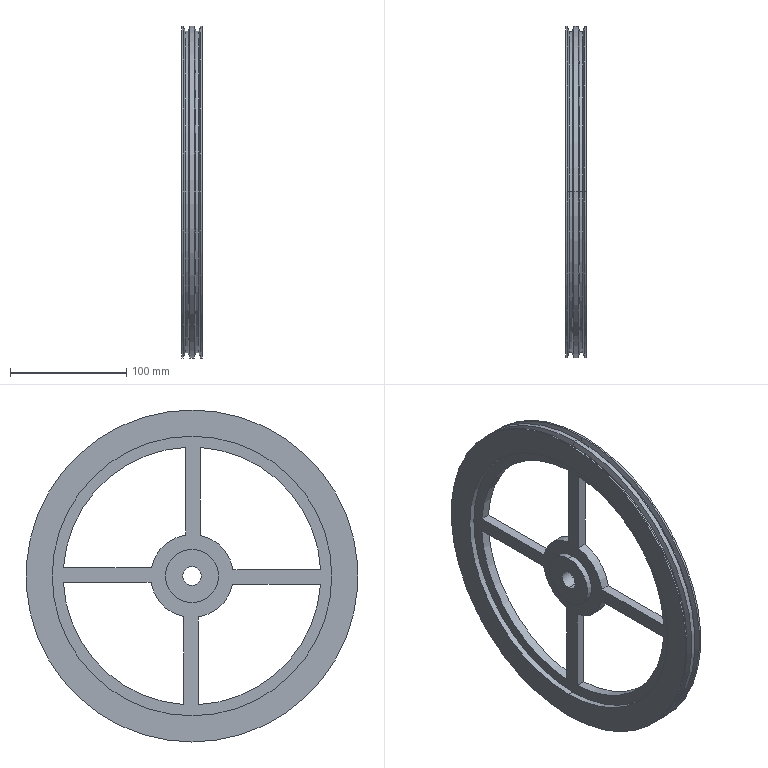Part | SolidWorks | features ICE 6, CirPattern 1, Revolution 1 | 1 solid | 50 faces | box 18 x 285 x 285 mm | volume 431975 mm3 | cylinder 28 | plane 14 | cone 8 | commonest cylinder face diameters 285 x6 45.741 x4 71.176 x4 221.11 x4 240 x4 276.214 x4
STEP:
#1=CARTESIAN_POINT('',(0.,0.,22.87));
#2=VERTEX_POINT('',#1);
#3=CARTESIAN_POINT('',(0.,0.,-22.87));
#4=VERTEX_POINT('',#3);
#5=CARTESIAN_POINT('',(0.,0.,0.));
#6=DIRECTION('',(-1.,0.,0.));
#7=DIRECTION('',(0.,0.,1.));
#8=AXIS2_PLACEMENT_3D('',#5,#6,#7);
#9=CIRCLE('',#8,22.87);
#10=EDGE_CURVE('',#2,#4,#9,.T.);
#11=ORIENTED_EDGE('',*,*,#10,.F.);
#12=CARTESIAN_POINT('',(5.,0.,22.87));
#13=VERTEX_POINT('',#12);
#14=CARTESIAN_POINT('',(0.,0.,22.87));
#15=DIRECTION('',(1.,0.,0.));
#16=VECTOR('',#15,1000.);
#17=LINE('',#14,#16);
#18=EDGE_CURVE('',#2,#13,#17,.T.);
#19=ORIENTED_EDGE('',*,*,#18,.T.);
#20=CARTESIAN_POINT('',(5.,0.,-22.87));
#21=VERTEX_POINT('',#20);
#22=CARTESIAN_POINT('',(5.,0.,0.));
#23=DIRECTION('',(-1.,0.,0.));
#24=DIRECTION('',(0.,0.,1.));
#25=AXIS2_PLACEMENT_3D('',#22,#23,#24);
#26=CIRCLE('',#25,22.87);
#27=EDGE_CURVE('',#13,#21,#26,.T.);
#28=ORIENTED_EDGE('',*,*,#27,.T.);
#29=CARTESIAN_POINT('',(0.,0.,-22.87));
#30=DIRECTION('',(1.,0.,0.));
#31=VECTOR('',#30,1000.);
#32=LINE('',#29,#31);
#33=EDGE_CURVE('',#4,#21,#32,.T.);
#34=ORIENTED_EDGE('',*,*,#33,.F.);
#35=EDGE_LOOP('',(#11,#19,#28,#34));
#36=FACE_OUTER_BOUND('',#35,.T.);
#37=CARTESIAN_POINT('',(0.,0.,0.));
#38=DIRECTION('',(1.,0.,0.));
#39=DIRECTION('',(0.,0.,-1.));
#40=AXIS2_PLACEMENT_3D('',#37,#38,#39);
#41=CYLINDRICAL_SURFACE('',#40,22.87);
#42=ADVANCED_FACE('',(#36),#41,.T.);
#43=CARTESIAN_POINT('',(18.,0.,-22.87));
#44=VERTEX_POINT('',#43);
#45=CARTESIAN_POINT('',(18.,0.,22.87));
#46=VERTEX_POINT('',#45);
#47=CARTESIAN_POINT('',(18.,0.,0.));
#48=DIRECTION('',(1.,0.,0.));
#49=DIRECTION('',(0.,0.,-1.));
#50=AXIS2_PLACEMENT_3D('',#47,#48,#49);
#51=CIRCLE('',#50,22.87);
#52=EDGE_CURVE('',#44,#46,#51,.T.);
#53=ORIENTED_EDGE('',*,*,#52,.F.);
#54=CARTESIAN_POINT('',(13.,0.,-22.87));
#55=VERTEX_POINT('',#54);
#56=CARTESIAN_POINT('',(18.,0.,-22.87));
#57=DIRECTION('',(-1.,0.,0.));
#58=VECTOR('',#57,1000.);
#59=LINE('',#56,#58);
#60=EDGE_CURVE('',#44,#55,#59,.T.);
#61=ORIENTED_EDGE('',*,*,#60,.T.);
#62=CARTESIAN_POINT('',(13.,0.,22.87));
#63=VERTEX_POINT('',#62);
#64=CARTESIAN_POINT('',(13.,0.,0.));
#65=DIRECTION('',(1.,0.,0.));
#66=DIRECTION('',(0.,0.,-1.));
#67=AXIS2_PLACEMENT_3D('',#64,#65,#66);
#68=CIRCLE('',#67,22.87);
#69=EDGE_CURVE('',#55,#63,#68,.T.);
#70=ORIENTED_EDGE('',*,*,#69,.T.);
#71=CARTESIAN_POINT('',(18.,0.,22.87));
#72=DIRECTION('',(-1.,0.,0.));
#73=VECTOR('',#72,1000.);
#74=LINE('',#71,#73);
#75=EDGE_CURVE('',#46,#63,#74,.T.);
#76=ORIENTED_EDGE('',*,*,#75,.F.);
#77=EDGE_LOOP('',(#53,#61,#70,#76));
#78=FACE_OUTER_BOUND('',#77,.T.);
#79=CARTESIAN_POINT('',(18.,0.,0.));
#80=DIRECTION('',(-1.,0.,0.));
#81=DIRECTION('',(0.,0.,1.));
#82=AXIS2_PLACEMENT_3D('',#79,#80,#81);
#83=CYLINDRICAL_SURFACE('',#82,22.87);
#84=ADVANCED_FACE('',(#78),#83,.T.);
#85=CARTESIAN_POINT('',(0.,0.,-8.));
#86=VERTEX_POINT('',#85);
#87=CARTESIAN_POINT('',(0.,0.,8.));
#88=VERTEX_POINT('',#87);
#89=CARTESIAN_POINT('',(0.,0.,0.));
#90=DIRECTION('',(-1.,0.,0.));
#91=DIRECTION('',(0.,0.,1.));
#92=AXIS2_PLACEMENT_3D('',#89,#90,#91);
#93=CIRCLE('',#92,8.);
#94=EDGE_CURVE('',#86,#88,#93,.T.);
#95=ORIENTED_EDGE('',*,*,#94,.T.);
#96=CARTESIAN_POINT('',(18.,0.,8.));
#97=VERTEX_POINT('',#96);
#98=CARTESIAN_POINT('',(0.,0.,8.));
#99=DIRECTION('',(1.,0.,0.));
#100=VECTOR('',#99,1000.);
#101=LINE('',#98,#100);
#102=EDGE_CURVE('',#88,#97,#101,.T.);
#103=ORIENTED_EDGE('',*,*,#102,.T.);
#104=CARTESIAN_POINT('',(18.,0.,-8.));
#105=VERTEX_POINT('',#104);
#106=CARTESIAN_POINT('',(18.,0.,0.));
#107=DIRECTION('',(1.,0.,0.));
#108=DIRECTION('',(0.,0.,-1.));
#109=AXIS2_PLACEMENT_3D('',#106,#107,#108);
#110=CIRCLE('',#109,8.);
#111=EDGE_CURVE('',#97,#105,#110,.T.);
#112=ORIENTED_EDGE('',*,*,#111,.T.);
#113=CARTESIAN_POINT('',(0.,0.,-8.));
#114=DIRECTION('',(1.,0.,0.));
#115=VECTOR('',#114,1000.);
#116=LINE('',#113,#115);
#117=EDGE_CURVE('',#86,#105,#116,.T.);
#118=ORIENTED_EDGE('',*,*,#117,.F.);
#119=EDGE_LOOP('',(#95,#103,#112,#118));
#120=FACE_OUTER_BOUND('',#119,.T.);
#121=CARTESIAN_POINT('',(0.,0.,0.));
#122=DIRECTION('',(1.,0.,0.));
#123=DIRECTION('',(0.,0.,-1.));
#124=AXIS2_PLACEMENT_3D('',#121,#122,#123);
#125=CYLINDRICAL_SURFACE('',#124,8.);
#126=ADVANCED_FACE('',(#120),#125,.F.);
#127=CARTESIAN_POINT('',(13.,0.,120.));
#128=VERTEX_POINT('',#127);
#129=CARTESIAN_POINT('',(13.,0.,-120.));
#130=VERTEX_POINT('',#129);
#131=CARTESIAN_POINT('',(13.,0.,0.));
#132=DIRECTION('',(1.,0.,0.));
#133=DIRECTION('',(0.,0.,-1.));
#134=AXIS2_PLACEMENT_3D('',#131,#132,#133);
#135=CIRCLE('',#134,120.);
#136=EDGE_CURVE('',#128,#130,#135,.T.);
#137=ORIENTED_EDGE('',*,*,#136,.F.);
#138=CARTESIAN_POINT('',(18.,0.,120.));
#139=VERTEX_POINT('',#138);
#140=CARTESIAN_POINT('',(13.,0.,120.));
#141=DIRECTION('',(1.,0.,0.));
#142=VECTOR('',#141,1000.);
#143=LINE('',#140,#142);
#144=EDGE_CURVE('',#128,#139,#143,.T.);
#145=ORIENTED_EDGE('',*,*,#144,.T.);
#146=CARTESIAN_POINT('',(18.,0.,-120.));
#147=VERTEX_POINT('',#146);
#148=CARTESIAN_POINT('',(18.,0.,0.));
#149=DIRECTION('',(1.,0.,0.));
#150=DIRECTION('',(0.,0.,-1.));
#151=AXIS2_PLACEMENT_3D('',#148,#149,#150);
#152=CIRCLE('',#151,120.);
#153=EDGE_CURVE('',#139,#147,#152,.T.);
#154=ORIENTED_EDGE('',*,*,#153,.T.);
#155=CARTESIAN_POINT('',(13.,0.,-120.));
#156=DIRECTION('',(1.,0.,0.));
#157=VECTOR('',#156,1000.);
#158=LINE('',#155,#157);
#159=EDGE_CURVE('',#130,#147,#158,.T.);
#160=ORIENTED_EDGE('',*,*,#159,.F.);
#161=EDGE_LOOP('',(#137,#145,#154,#160));
#162=FACE_OUTER_BOUND('',#161,.T.);
#163=CARTESIAN_POINT('',(13.,0.,0.));
#164=DIRECTION('',(1.,0.,0.));
#165=DIRECTION('',(0.,0.,-1.));
#166=AXIS2_PLACEMENT_3D('',#163,#164,#165);
#167=CYLINDRICAL_SURFACE('',#166,120.);
#168=ADVANCED_FACE('',(#162),#167,.F.);
#169=CARTESIAN_POINT('',(5.,0.,-120.));
#170=VERTEX_POINT('',#169);
#171=CARTESIAN_POINT('',(5.,0.,120.));
#172=VERTEX_POINT('',#171);
#173=CARTESIAN_POINT('',(5.,0.,0.));
#174=DIRECTION('',(-1.,0.,0.));
#175=DIRECTION('',(0.,0.,1.));
#176=AXIS2_PLACEMENT_3D('',#173,#174,#175);
#177=CIRCLE('',#176,120.);
#178=EDGE_CURVE('',#170,#172,#177,.T.);
#179=ORIENTED_EDGE('',*,*,#178,.F.);
#180=CARTESIAN_POINT('',(0.,0.,-120.));
#181=VERTEX_POINT('',#180);
#182=CARTESIAN_POINT('',(5.,0.,-120.));
#183=DIRECTION('',(-1.,0.,0.));
#184=VECTOR('',#183,1000.);
#185=LINE('',#182,#184);
#186=EDGE_CURVE('',#170,#181,#185,.T.);
#187=ORIENTED_EDGE('',*,*,#186,.T.);
#188=CARTESIAN_POINT('',(0.,0.,120.));
#189=VERTEX_POINT('',#188);
#190=CARTESIAN_POINT('',(0.,0.,0.));
#191=DIRECTION('',(-1.,0.,0.));
#192=DIRECTION('',(0.,0.,1.));
#193=AXIS2_PLACEMENT_3D('',#190,#191,#192);
#194=CIRCLE('',#193,120.);
#195=EDGE_CURVE('',#181,#189,#194,.T.);
#196=ORIENTED_EDGE('',*,*,#195,.T.);
#197=CARTESIAN_POINT('',(5.,0.,120.));
#198=DIRECTION('',(-1.,0.,0.));
#199=VECTOR('',#198,1000.);
#200=LINE('',#197,#199);
#201=EDGE_CURVE('',#172,#189,#200,.T.);
#202=ORIENTED_EDGE('',*,*,#201,.F.);
#203=EDGE_LOOP('',(#179,#187,#196,#202));
#204=FACE_OUTER_BOUND('',#203,.T.);
#205=CARTESIAN_POINT('',(5.,0.,0.));
#206=DIRECTION('',(-1.,0.,0.));
#207=DIRECTION('',(0.,0.,1.));
#208=AXIS2_PLACEMENT_3D('',#205,#206,#207);
#209=CYLINDRICAL_SURFACE('',#208,120.);
#210=ADVANCED_FACE('',(#204),#209,.F.);
#211=CARTESIAN_POINT('',(18.,0.,142.5));
#212=VERTEX_POINT('',#211);
#213=CARTESIAN_POINT('',(18.,0.,-142.5));
#214=VERTEX_POINT('',#213);
#215=CARTESIAN_POINT('',(18.,0.,0.));
#216=DIRECTION('',(-1.,0.,0.));
#217=DIRECTION('',(0.,0.,1.));
#218=AXIS2_PLACEMENT_3D('',#215,#216,#217);
#219=CIRCLE('',#218,142.5);
#220=EDGE_CURVE('',#212,#214,#219,.T.);
#221=ORIENTED_EDGE('',*,*,#220,.T.);
#222=CARTESIAN_POINT('',(16.241,0.,-142.5));
#223=VERTEX_POINT('',#222);
#224=CARTESIAN_POINT('',(0.,0.,-142.5));
#225=DIRECTION('',(-1.,0.,0.));
#226=VECTOR('',#225,1000.);
#227=LINE('',#224,#226);
#228=EDGE_CURVE('',#214,#223,#227,.T.);
#229=ORIENTED_EDGE('',*,*,#228,.T.);
#230=CARTESIAN_POINT('',(16.241,0.,142.5));
#231=VERTEX_POINT('',#230);
#232=CARTESIAN_POINT('',(16.241,0.,0.));
#233=DIRECTION('',(-1.,0.,0.));
#234=DIRECTION('',(0.,0.,1.));
#235=AXIS2_PLACEMENT_3D('',#232,#233,#234);
#236=CIRCLE('',#235,142.5);
#237=EDGE_CURVE('',#231,#223,#236,.T.);
#238=ORIENTED_EDGE('',*,*,#237,.F.);
#239=CARTESIAN_POINT('',(0.,0.,142.5));
#240=DIRECTION('',(-1.,0.,0.));
#241=VECTOR('',#240,1000.);
#242=LINE('',#239,#241);
#243=EDGE_CURVE('',#212,#231,#242,.T.);
#244=ORIENTED_EDGE('',*,*,#243,.F.);
#245=EDGE_LOOP('',(#221,#229,#238,#244));
#246=FACE_OUTER_BOUND('',#245,.T.);
#247=CARTESIAN_POINT('',(0.,0.,0.));
#248=DIRECTION('',(-1.,0.,0.));
#249=DIRECTION('',(0.,0.,1.));
#250=AXIS2_PLACEMENT_3D('',#247,#248,#249);
#251=CYLINDRICAL_SURFACE('',#250,142.5);
#252=ADVANCED_FACE('',(#246),#251,.T.);
#253=CARTESIAN_POINT('',(14.915,0.,138.107));
#254=VERTEX_POINT('',#253);
#255=CARTESIAN_POINT('',(14.915,0.,-138.107));
#256=VERTEX_POINT('',#255);
#257=CARTESIAN_POINT('',(14.915,0.,0.));
#258=DIRECTION('',(-1.,0.,0.));
#259=DIRECTION('',(0.,0.,1.));
#260=AXIS2_PLACEMENT_3D('',#257,#258,#259);
#261=CIRCLE('',#260,138.107);
#262=EDGE_CURVE('',#254,#256,#261,.T.);
#263=ORIENTED_EDGE('',*,*,#262,.F.);
#264=CARTESIAN_POINT('',(16.241,0.,142.5));
#265=DIRECTION('',(0.2889,0.,0.9574));
#266=VECTOR('',#265,1000.);
#267=LINE('',#264,#266);
#268=EDGE_CURVE('',#254,#231,#267,.T.);
#269=ORIENTED_EDGE('',*,*,#268,.T.);
#270=ORIENTED_EDGE('',*,*,#237,.T.);
#271=CARTESIAN_POINT('',(16.241,0.,-142.5));
#272=DIRECTION('',(0.2889,0.,-0.9574));
#273=VECTOR('',#272,1000.);
#274=LINE('',#271,#273);
#275=EDGE_CURVE('',#256,#223,#274,.T.);
#276=ORIENTED_EDGE('',*,*,#275,.F.);
#277=EDGE_LOOP('',(#263,#269,#270,#276));
#278=FACE_OUTER_BOUND('',#277,.T.);
#279=CARTESIAN_POINT('',(16.241,0.,0.));
#280=DIRECTION('',(1.,0.,0.));
#281=DIRECTION('',(0.,0.,-1.));
#282=AXIS2_PLACEMENT_3D('',#279,#280,#281);
#283=CONICAL_SURFACE('',#282,142.5,1.278);
#284=ADVANCED_FACE('',(#278),#283,.T.);
#285=ORIENTED_EDGE('',*,*,#262,.T.);
#286=CARTESIAN_POINT('',(12.264,0.,-138.107));
#287=VERTEX_POINT('',#286);
#288=CARTESIAN_POINT('',(0.,0.,-138.107));
#289=DIRECTION('',(-1.,0.,0.));
#290=VECTOR('',#289,1000.);
#291=LINE('',#288,#290);
#292=EDGE_CURVE('',#256,#287,#291,.T.);
#293=ORIENTED_EDGE('',*,*,#292,.T.);
#294=CARTESIAN_POINT('',(12.264,0.,138.107));
#295=VERTEX_POINT('',#294);
#296=CARTESIAN_POINT('',(12.264,0.,0.));
#297=DIRECTION('',(-1.,0.,0.));
#298=DIRECTION('',(0.,0.,1.));
#299=AXIS2_PLACEMENT_3D('',#296,#297,#298);
#300=CIRCLE('',#299,138.107);
#301=EDGE_CURVE('',#295,#287,#300,.T.);
#302=ORIENTED_EDGE('',*,*,#301,.F.);
#303=CARTESIAN_POINT('',(0.,0.,138.107));
#304=DIRECTION('',(-1.,0.,0.));
#305=VECTOR('',#304,1000.);
#306=LINE('',#303,#305);
#307=EDGE_CURVE('',#254,#295,#306,.T.);
#308=ORIENTED_EDGE('',*,*,#307,.F.);
#309=EDGE_LOOP('',(#285,#293,#302,#308));
#310=FACE_OUTER_BOUND('',#309,.T.);
#311=CARTESIAN_POINT('',(0.,0.,0.));
#312=DIRECTION('',(-1.,0.,0.));
#313=DIRECTION('',(0.,0.,1.));
#314=AXIS2_PLACEMENT_3D('',#311,#312,#313);
#315=CYLINDRICAL_SURFACE('',#314,138.107);
#316=ADVANCED_FACE('',(#310),#315,.T.);
#317=ORIENTED_EDGE('',*,*,#301,.T.);
#318=CARTESIAN_POINT('',(11.013,0.,-142.5));
#319=VERTEX_POINT('',#318);
#320=CARTESIAN_POINT('',(12.264,0.,-138.107));
#321=DIRECTION('',(-0.2741,0.,-0.9617));
#322=VECTOR('',#321,1000.);
#323=LINE('',#320,#322);
#324=EDGE_CURVE('',#287,#319,#323,.T.);
#325=ORIENTED_EDGE('',*,*,#324,.T.);
#326=CARTESIAN_POINT('',(11.013,0.,142.5));
#327=VERTEX_POINT('',#326);
#328=CARTESIAN_POINT('',(11.013,0.,0.));
#329=DIRECTION('',(-1.,0.,0.));
#330=DIRECTION('',(0.,0.,1.));
#331=AXIS2_PLACEMENT_3D('',#328,#329,#330);
#332=CIRCLE('',#331,142.5);
#333=EDGE_CURVE('',#327,#319,#332,.T.);
#334=ORIENTED_EDGE('',*,*,#333,.F.);
#335=CARTESIAN_POINT('',(12.264,0.,138.107));
#336=DIRECTION('',(-0.2741,0.,0.9617));
#337=VECTOR('',#336,1000.);
#338=LINE('',#335,#337);
#339=EDGE_CURVE('',#295,#327,#338,.T.);
#340=ORIENTED_EDGE('',*,*,#339,.F.);
#341=EDGE_LOOP('',(#317,#325,#334,#340));
#342=FACE_OUTER_BOUND('',#341,.T.);
#343=CARTESIAN_POINT('',(12.264,0.,0.));
#344=DIRECTION('',(-1.,0.,0.));
#345=DIRECTION('',(0.,0.,1.));
#346=AXIS2_PLACEMENT_3D('',#343,#344,#345);
#347=CONICAL_SURFACE('',#346,138.107,1.293);
#348=ADVANCED_FACE('',(#342),#347,.T.);
#349=ORIENTED_EDGE('',*,*,#333,.T.);
#350=CARTESIAN_POINT('',(7.11,0.,-142.5));
#351=VERTEX_POINT('',#350);
#352=CARTESIAN_POINT('',(0.,0.,-142.5));
#353=DIRECTION('',(-1.,0.,0.));
#354=VECTOR('',#353,1000.);
#355=LINE('',#352,#354);
#356=EDGE_CURVE('',#319,#351,#355,.T.);
#357=ORIENTED_EDGE('',*,*,#356,.T.);
#358=CARTESIAN_POINT('',(7.11,0.,142.5));
#359=VERTEX_POINT('',#358);
#360=CARTESIAN_POINT('',(7.11,0.,0.));
#361=DIRECTION('',(-1.,0.,0.));
#362=DIRECTION('',(0.,0.,1.));
#363=AXIS2_PLACEMENT_3D('',#360,#361,#362);
#364=CIRCLE('',#363,142.5);
#365=EDGE_CURVE('',#359,#351,#364,.T.);
#366=ORIENTED_EDGE('',*,*,#365,.F.);
#367=CARTESIAN_POINT('',(0.,0.,142.5));
#368=DIRECTION('',(-1.,0.,0.));
#369=VECTOR('',#368,1000.);
#370=LINE('',#367,#369);
#371=EDGE_CURVE('',#327,#359,#370,.T.);
#372=ORIENTED_EDGE('',*,*,#371,.F.);
#373=EDGE_LOOP('',(#349,#357,#366,#372));
#374=FACE_OUTER_BOUND('',#373,.T.);
#375=CARTESIAN_POINT('',(0.,0.,0.));
#376=DIRECTION('',(-1.,0.,0.));
#377=DIRECTION('',(0.,0.,1.));
#378=AXIS2_PLACEMENT_3D('',#375,#376,#377);
#379=CYLINDRICAL_SURFACE('',#378,142.5);
#380=ADVANCED_FACE('',(#374),#379,.T.);
#381=CARTESIAN_POINT('',(5.784,0.,138.107));
#382=VERTEX_POINT('',#381);
#383=CARTESIAN_POINT('',(5.784,0.,-138.107));
#384=VERTEX_POINT('',#383);
#385=CARTESIAN_POINT('',(5.784,0.,0.));
#386=DIRECTION('',(-1.,0.,0.));
#387=DIRECTION('',(0.,0.,1.));
#388=AXIS2_PLACEMENT_3D('',#385,#386,#387);
#389=CIRCLE('',#388,138.107);
#390=EDGE_CURVE('',#382,#384,#389,.T.);
#391=ORIENTED_EDGE('',*,*,#390,.F.);
#392=CARTESIAN_POINT('',(7.11,0.,142.5));
#393=DIRECTION('',(0.2889,0.,0.9574));
#394=VECTOR('',#393,1000.);
#395=LINE('',#392,#394);
#396=EDGE_CURVE('',#382,#359,#395,.T.);
#397=ORIENTED_EDGE('',*,*,#396,.T.);
#398=ORIENTED_EDGE('',*,*,#365,.T.);
#399=CARTESIAN_POINT('',(7.11,0.,-142.5));
#400=DIRECTION('',(0.2889,0.,-0.9574));
#401=VECTOR('',#400,1000.);
#402=LINE('',#399,#401);
#403=EDGE_CURVE('',#384,#351,#402,.T.);
#404=ORIENTED_EDGE('',*,*,#403,.F.);
#405=EDGE_LOOP('',(#391,#397,#398,#404));
#406=FACE_OUTER_BOUND('',#405,.T.);
#407=CARTESIAN_POINT('',(7.11,0.,0.));
#408=DIRECTION('',(1.,0.,0.));
#409=DIRECTION('',(0.,0.,-1.));
#410=AXIS2_PLACEMENT_3D('',#407,#408,#409);
#411=CONICAL_SURFACE('',#410,142.5,1.278);
#412=ADVANCED_FACE('',(#406),#411,.T.);
#413=ORIENTED_EDGE('',*,*,#390,.T.);
#414=CARTESIAN_POINT('',(3.207,0.,-138.107));
#415=VERTEX_POINT('',#414);
#416=CARTESIAN_POINT('',(0.,0.,-138.107));
#417=DIRECTION('',(-1.,0.,0.));
#418=VECTOR('',#417,1000.);
#419=LINE('',#416,#418);
#420=EDGE_CURVE('',#384,#415,#419,.T.);
#421=ORIENTED_EDGE('',*,*,#420,.T.);
#422=CARTESIAN_POINT('',(3.207,0.,138.107));
#423=VERTEX_POINT('',#422);
#424=CARTESIAN_POINT('',(3.207,0.,0.));
#425=DIRECTION('',(-1.,0.,0.));
#426=DIRECTION('',(0.,0.,1.));
#427=AXIS2_PLACEMENT_3D('',#424,#425,#426);
#428=CIRCLE('',#427,138.107);
#429=EDGE_CURVE('',#423,#415,#428,.T.);
#430=ORIENTED_EDGE('',*,*,#429,.F.);
#431=CARTESIAN_POINT('',(0.,0.,138.107));
#432=DIRECTION('',(-1.,0.,0.));
#433=VECTOR('',#432,1000.);
#434=LINE('',#431,#433);
#435=EDGE_CURVE('',#382,#423,#434,.T.);
#436=ORIENTED_EDGE('',*,*,#435,.F.);
#437=EDGE_LOOP('',(#413,#421,#430,#436));
#438=FACE_OUTER_BOUND('',#437,.T.);
#439=CARTESIAN_POINT('',(0.,0.,0.));
#440=DIRECTION('',(-1.,0.,0.));
#441=DIRECTION('',(0.,0.,1.));
#442=AXIS2_PLACEMENT_3D('',#439,#440,#441);
#443=CYLINDRICAL_SURFACE('',#442,138.107);
#444=ADVANCED_FACE('',(#438),#443,.T.);
#445=ORIENTED_EDGE('',*,*,#429,.T.);
#446=CARTESIAN_POINT('',(1.44,0.,-142.5));
#447=VERTEX_POINT('',#446);
#448=CARTESIAN_POINT('',(3.207,0.,-138.107));
#449=DIRECTION('',(-0.3732,0.,-0.9277));
#450=VECTOR('',#449,1000.);
#451=LINE('',#448,#450);
#452=EDGE_CURVE('',#415,#447,#451,.T.);
#453=ORIENTED_EDGE('',*,*,#452,.T.);
#454=CARTESIAN_POINT('',(1.44,0.,142.5));
#455=VERTEX_POINT('',#454);
#456=CARTESIAN_POINT('',(1.44,0.,0.));
#457=DIRECTION('',(-1.,0.,0.));
#458=DIRECTION('',(0.,0.,1.));
#459=AXIS2_PLACEMENT_3D('',#456,#457,#458);
#460=CIRCLE('',#459,142.5);
#461=EDGE_CURVE('',#455,#447,#460,.T.);
#462=ORIENTED_EDGE('',*,*,#461,.F.);
#463=CARTESIAN_POINT('',(3.207,0.,138.107));
#464=DIRECTION('',(-0.3732,0.,0.9277));
#465=VECTOR('',#464,1000.);
#466=LINE('',#463,#465);
#467=EDGE_CURVE('',#423,#455,#466,.T.);
#468=ORIENTED_EDGE('',*,*,#467,.F.);
#469=EDGE_LOOP('',(#445,#453,#462,#468));
#470=FACE_OUTER_BOUND('',#469,.T.);
#471=CARTESIAN_POINT('',(3.207,0.,0.));
#472=DIRECTION('',(-1.,0.,0.));
#473=DIRECTION('',(0.,0.,1.));
#474=AXIS2_PLACEMENT_3D('',#471,#472,#473);
#475=CONICAL_SURFACE('',#474,138.107,1.188);
#476=ADVANCED_FACE('',(#470),#475,.T.);
#477=ORIENTED_EDGE('',*,*,#461,.T.);
#478=CARTESIAN_POINT('',(0.,0.,-142.5));
#479=VERTEX_POINT('',#478);
#480=CARTESIAN_POINT('',(0.,0.,-142.5));
#481=DIRECTION('',(-1.,0.,0.));
#482=VECTOR('',#481,1000.);
#483=LINE('',#480,#482);
#484=EDGE_CURVE('',#447,#479,#483,.T.);
#485=ORIENTED_EDGE('',*,*,#484,.T.);
#486=CARTESIAN_POINT('',(0.,0.,142.5));
#487=VERTEX_POINT('',#486);
#488=CARTESIAN_POINT('',(0.,0.,0.));
#489=DIRECTION('',(-1.,0.,0.));
#490=DIRECTION('',(0.,0.,1.));
#491=AXIS2_PLACEMENT_3D('',#488,#489,#490);
#492=CIRCLE('',#491,142.5);
#493=EDGE_CURVE('',#487,#479,#492,.T.);
#494=ORIENTED_EDGE('',*,*,#493,.F.);
#495=CARTESIAN_POINT('',(0.,0.,142.5));
#496=DIRECTION('',(-1.,0.,0.));
#497=VECTOR('',#496,1000.);
#498=LINE('',#495,#497);
#499=EDGE_CURVE('',#455,#487,#498,.T.);
#500=ORIENTED_EDGE('',*,*,#499,.F.);
#501=EDGE_LOOP('',(#477,#485,#494,#500));
#502=FACE_OUTER_BOUND('',#501,.T.);
#503=CARTESIAN_POINT('',(0.,0.,0.));
#504=DIRECTION('',(-1.,0.,0.));
#505=DIRECTION('',(0.,0.,1.));
#506=AXIS2_PLACEMENT_3D('',#503,#504,#505);
#507=CYLINDRICAL_SURFACE('',#506,142.5);
#508=ADVANCED_FACE('',(#502),#507,.T.);
#509=CARTESIAN_POINT('',(5.,-7.038,34.885));
#510=VERTEX_POINT('',#509);
#511=CARTESIAN_POINT('',(5.,-35.176,5.402));
#512=VERTEX_POINT('',#511);
#513=CARTESIAN_POINT('',(5.,0.,0.));
#514=DIRECTION('',(1.,0.,0.));
#515=DIRECTION('',(0.,0.,-1.));
#516=AXIS2_PLACEMENT_3D('',#513,#514,#515);
#517=CIRCLE('',#516,35.588);
#518=EDGE_CURVE('',#510,#512,#517,.T.);
#519=ORIENTED_EDGE('',*,*,#518,.F.);
#520=CARTESIAN_POINT('',(5.,-7.038,110.331));
#521=VERTEX_POINT('',#520);
#522=CARTESIAN_POINT('',(5.,-7.038,34.885));
#523=DIRECTION('',(0.,0.,-1.));
#524=VECTOR('',#523,1000.);
#525=LINE('',#522,#524);
#526=EDGE_CURVE('',#521,#510,#525,.T.);
#527=ORIENTED_EDGE('',*,*,#526,.F.);
#528=CARTESIAN_POINT('',(5.,-110.423,5.402));
#529=VERTEX_POINT('',#528);
#530=CARTESIAN_POINT('',(5.,0.,0.));
#531=DIRECTION('',(-1.,0.,0.));
#532=DIRECTION('',(0.,0.,-1.));
#533=AXIS2_PLACEMENT_3D('',#530,#531,#532);
#534=CIRCLE('',#533,110.555);
#535=EDGE_CURVE('',#529,#521,#534,.T.);
#536=ORIENTED_EDGE('',*,*,#535,.F.);
#537=CARTESIAN_POINT('',(5.,-35.176,5.402));
#538=DIRECTION('',(0.,-1.,0.));
#539=VECTOR('',#538,1000.);
#540=LINE('',#537,#539);
#541=EDGE_CURVE('',#512,#529,#540,.T.);
#542=ORIENTED_EDGE('',*,*,#541,.F.);
#543=EDGE_LOOP('',(#519,#527,#536,#542));
#544=FACE_BOUND('',#543,.T.);
#545=CARTESIAN_POINT('',(5.,34.885,7.038));
#546=VERTEX_POINT('',#545);
#547=CARTESIAN_POINT('',(5.,5.402,35.176));
#548=VERTEX_POINT('',#547);
#549=CARTESIAN_POINT('',(5.,0.,0.));
#550=DIRECTION('',(1.,0.,0.));
#551=DIRECTION('',(0.,-1.,0.));
#552=AXIS2_PLACEMENT_3D('',#549,#550,#551);
#553=CIRCLE('',#552,35.588);
#554=EDGE_CURVE('',#546,#548,#553,.T.);
#555=ORIENTED_EDGE('',*,*,#554,.F.);
#556=CARTESIAN_POINT('',(5.,110.331,7.038));
#557=VERTEX_POINT('',#556);
#558=CARTESIAN_POINT('',(5.,34.885,7.038));
#559=DIRECTION('',(0.,-1.,0.));
#560=VECTOR('',#559,1000.);
#561=LINE('',#558,#560);
#562=EDGE_CURVE('',#557,#546,#561,.T.);
#563=ORIENTED_EDGE('',*,*,#562,.F.);
#564=CARTESIAN_POINT('',(5.,5.402,110.423));
#565=VERTEX_POINT('',#564);
#566=CARTESIAN_POINT('',(5.,0.,0.));
#567=DIRECTION('',(-1.,0.,0.));
#568=DIRECTION('',(0.,-1.,0.));
#569=AXIS2_PLACEMENT_3D('',#566,#567,#568);
#570=CIRCLE('',#569,110.555);
#571=EDGE_CURVE('',#565,#557,#570,.T.);
#572=ORIENTED_EDGE('',*,*,#571,.F.);
#573=CARTESIAN_POINT('',(5.,5.402,35.176));
#574=DIRECTION('',(0.,0.,1.));
#575=VECTOR('',#574,1000.);
#576=LINE('',#573,#575);
#577=EDGE_CURVE('',#548,#565,#576,.T.);
#578=ORIENTED_EDGE('',*,*,#577,.F.);
#579=EDGE_LOOP('',(#555,#563,#572,#578));
#580=FACE_BOUND('',#579,.T.);
#581=CARTESIAN_POINT('',(5.,-34.885,-7.038));
#582=VERTEX_POINT('',#581);
#583=CARTESIAN_POINT('',(5.,-5.402,-35.176));
#584=VERTEX_POINT('',#583);
#585=CARTESIAN_POINT('',(5.,0.,0.));
#586=DIRECTION('',(1.,0.,0.));
#587=DIRECTION('',(0.,1.,0.));
#588=AXIS2_PLACEMENT_3D('',#585,#586,#587);
#589=CIRCLE('',#588,35.588);
#590=EDGE_CURVE('',#582,#584,#589,.T.);
#591=ORIENTED_EDGE('',*,*,#590,.F.);
#592=CARTESIAN_POINT('',(5.,-110.331,-7.038));
#593=VERTEX_POINT('',#592);
#594=CARTESIAN_POINT('',(5.,-34.885,-7.038));
#595=DIRECTION('',(0.,1.,0.));
#596=VECTOR('',#595,1000.);
#597=LINE('',#594,#596);
#598=EDGE_CURVE('',#593,#582,#597,.T.);
#599=ORIENTED_EDGE('',*,*,#598,.F.);
#600=CARTESIAN_POINT('',(5.,-5.402,-110.423));
#601=VERTEX_POINT('',#600);
#602=CARTESIAN_POINT('',(5.,0.,0.));
#603=DIRECTION('',(-1.,0.,0.));
#604=DIRECTION('',(0.,1.,0.));
#605=AXIS2_PLACEMENT_3D('',#602,#603,#604);
#606=CIRCLE('',#605,110.555);
#607=EDGE_CURVE('',#601,#593,#606,.T.);
#608=ORIENTED_EDGE('',*,*,#607,.F.);
#609=CARTESIAN_POINT('',(5.,-5.402,-35.176));
#610=DIRECTION('',(0.,0.,-1.));
#611=VECTOR('',#610,1000.);
#612=LINE('',#609,#611);
#613=EDGE_CURVE('',#584,#601,#612,.T.);
#614=ORIENTED_EDGE('',*,*,#613,.F.);
#615=EDGE_LOOP('',(#591,#599,#608,#614));
#616=FACE_BOUND('',#615,.T.);
#617=CARTESIAN_POINT('',(5.,7.038,-34.885));
#618=VERTEX_POINT('',#617);
#619=CARTESIAN_POINT('',(5.,35.176,-5.402));
#620=VERTEX_POINT('',#619);
#621=CARTESIAN_POINT('',(5.,0.,0.));
#622=DIRECTION('',(1.,0.,0.));
#623=DIRECTION('',(0.,0.,1.));
#624=AXIS2_PLACEMENT_3D('',#621,#622,#623);
#625=CIRCLE('',#624,35.588);
#626=EDGE_CURVE('',#618,#620,#625,.T.);
#627=ORIENTED_EDGE('',*,*,#626,.F.);
#628=CARTESIAN_POINT('',(5.,7.038,-110.331));
#629=VERTEX_POINT('',#628);
#630=CARTESIAN_POINT('',(5.,7.038,-34.885));
#631=DIRECTION('',(0.,0.,1.));
#632=VECTOR('',#631,1000.);
#633=LINE('',#630,#632);
#634=EDGE_CURVE('',#629,#618,#633,.T.);
#635=ORIENTED_EDGE('',*,*,#634,.F.);
#636=CARTESIAN_POINT('',(5.,110.423,-5.402));
#637=VERTEX_POINT('',#636);
#638=CARTESIAN_POINT('',(5.,0.,0.));
#639=DIRECTION('',(-1.,0.,0.));
#640=DIRECTION('',(0.,0.,1.));
#641=AXIS2_PLACEMENT_3D('',#638,#639,#640);
#642=CIRCLE('',#641,110.555);
#643=EDGE_CURVE('',#637,#629,#642,.T.);
#644=ORIENTED_EDGE('',*,*,#643,.F.);
#645=CARTESIAN_POINT('',(5.,35.176,-5.402));
#646=DIRECTION('',(0.,1.,0.));
#647=VECTOR('',#646,1000.);
#648=LINE('',#645,#647);
#649=EDGE_CURVE('',#620,#637,#648,.T.);
#650=ORIENTED_EDGE('',*,*,#649,.F.);
#651=EDGE_LOOP('',(#627,#635,#644,#650));
#652=FACE_BOUND('',#651,.T.);
#653=CARTESIAN_POINT('',(5.,0.,0.));
#654=DIRECTION('',(-1.,0.,0.));
#655=DIRECTION('',(0.,0.,1.));
#656=AXIS2_PLACEMENT_3D('',#653,#654,#655);
#657=CIRCLE('',#656,120.);
#658=EDGE_CURVE('',#172,#170,#657,.T.);
#659=ORIENTED_EDGE('',*,*,#658,.T.);
#660=ORIENTED_EDGE('',*,*,#178,.T.);
#661=EDGE_LOOP('',(#659,#660));
#662=FACE_OUTER_BOUND('',#661,.T.);
#663=CARTESIAN_POINT('',(5.,0.,0.));
#664=DIRECTION('',(-1.,0.,0.));
#665=DIRECTION('',(0.,0.,1.));
#666=AXIS2_PLACEMENT_3D('',#663,#664,#665);
#667=CIRCLE('',#666,22.87);
#668=EDGE_CURVE('',#21,#13,#667,.T.);
#669=ORIENTED_EDGE('',*,*,#668,.F.);
#670=ORIENTED_EDGE('',*,*,#27,.F.);
#671=EDGE_LOOP('',(#669,#670));
#672=FACE_BOUND('',#671,.T.);
#673=CARTESIAN_POINT('',(5.,0.,0.));
#674=DIRECTION('',(-1.,0.,0.));
#675=DIRECTION('',(0.,0.,1.));
#676=AXIS2_PLACEMENT_3D('',#673,#674,#675);
#677=PLANE('',#676);
#678=ADVANCED_FACE('',(#544,#580,#616,#652,#662,#672),#677,.T.);
#679=CARTESIAN_POINT('',(13.,-35.176,5.402));
#680=VERTEX_POINT('',#679);
#681=CARTESIAN_POINT('',(13.,-7.038,34.885));
#682=VERTEX_POINT('',#681);
#683=CARTESIAN_POINT('',(13.,0.,0.));
#684=DIRECTION('',(-1.,0.,0.));
#685=DIRECTION('',(0.,0.,-1.));
#686=AXIS2_PLACEMENT_3D('',#683,#684,#685);
#687=CIRCLE('',#686,35.588);
#688=EDGE_CURVE('',#680,#682,#687,.T.);
#689=ORIENTED_EDGE('',*,*,#688,.F.);
#690=CARTESIAN_POINT('',(13.,-110.423,5.402));
#691=VERTEX_POINT('',#690);
#692=CARTESIAN_POINT('',(13.,0.,5.402));
#693=DIRECTION('',(0.,1.,0.));
#694=VECTOR('',#693,1000.);
#695=LINE('',#692,#694);
#696=EDGE_CURVE('',#691,#680,#695,.T.);
#697=ORIENTED_EDGE('',*,*,#696,.F.);
#698=CARTESIAN_POINT('',(13.,-7.038,110.331));
#699=VERTEX_POINT('',#698);
#700=CARTESIAN_POINT('',(13.,0.,0.));
#701=DIRECTION('',(1.,0.,0.));
#702=DIRECTION('',(0.,0.,-1.));
#703=AXIS2_PLACEMENT_3D('',#700,#701,#702);
#704=CIRCLE('',#703,110.555);
#705=EDGE_CURVE('',#699,#691,#704,.T.);
#706=ORIENTED_EDGE('',*,*,#705,.F.);
#707=CARTESIAN_POINT('',(13.,-7.038,0.));
#708=DIRECTION('',(0.,0.,1.));
#709=VECTOR('',#708,1000.);
#710=LINE('',#707,#709);
#711=EDGE_CURVE('',#682,#699,#710,.T.);
#712=ORIENTED_EDGE('',*,*,#711,.F.);
#713=EDGE_LOOP('',(#689,#697,#706,#712));
#714=FACE_BOUND('',#713,.T.);
#715=CARTESIAN_POINT('',(13.,5.402,35.176));
#716=VERTEX_POINT('',#715);
#717=CARTESIAN_POINT('',(13.,34.885,7.038));
#718=VERTEX_POINT('',#717);
#719=CARTESIAN_POINT('',(13.,0.,0.));
#720=DIRECTION('',(-1.,0.,0.));
#721=DIRECTION('',(0.,0.,-1.));
#722=AXIS2_PLACEMENT_3D('',#719,#720,#721);
#723=CIRCLE('',#722,35.588);
#724=EDGE_CURVE('',#716,#718,#723,.T.);
#725=ORIENTED_EDGE('',*,*,#724,.F.);
#726=CARTESIAN_POINT('',(13.,5.402,110.423));
#727=VERTEX_POINT('',#726);
#728=CARTESIAN_POINT('',(13.,5.402,0.));
#729=DIRECTION('',(0.,0.,-1.));
#730=VECTOR('',#729,1000.);
#731=LINE('',#728,#730);
#732=EDGE_CURVE('',#727,#716,#731,.T.);
#733=ORIENTED_EDGE('',*,*,#732,.F.);
#734=CARTESIAN_POINT('',(13.,110.331,7.038));
#735=VERTEX_POINT('',#734);
#736=CARTESIAN_POINT('',(13.,0.,0.));
#737=DIRECTION('',(1.,0.,0.));
#738=DIRECTION('',(0.,0.,-1.));
#739=AXIS2_PLACEMENT_3D('',#736,#737,#738);
#740=CIRCLE('',#739,110.555);
#741=EDGE_CURVE('',#735,#727,#740,.T.);
#742=ORIENTED_EDGE('',*,*,#741,.F.);
#743=CARTESIAN_POINT('',(13.,0.,7.038));
#744=DIRECTION('',(0.,1.,0.));
#745=VECTOR('',#744,1000.);
#746=LINE('',#743,#745);
#747=EDGE_CURVE('',#718,#735,#746,.T.);
#748=ORIENTED_EDGE('',*,*,#747,.F.);
#749=EDGE_LOOP('',(#725,#733,#742,#748));
#750=FACE_BOUND('',#749,.T.);
#751=CARTESIAN_POINT('',(13.,-5.402,-35.176));
#752=VERTEX_POINT('',#751);
#753=CARTESIAN_POINT('',(13.,-34.885,-7.038));
#754=VERTEX_POINT('',#753);
#755=CARTESIAN_POINT('',(13.,0.,0.));
#756=DIRECTION('',(-1.,0.,0.));
#757=DIRECTION('',(0.,0.,-1.));
#758=AXIS2_PLACEMENT_3D('',#755,#756,#757);
#759=CIRCLE('',#758,35.588);
#760=EDGE_CURVE('',#752,#754,#759,.T.);
#761=ORIENTED_EDGE('',*,*,#760,.F.);
#762=CARTESIAN_POINT('',(13.,-5.402,-110.423));
#763=VERTEX_POINT('',#762);
#764=CARTESIAN_POINT('',(13.,-5.402,0.));
#765=DIRECTION('',(0.,0.,1.));
#766=VECTOR('',#765,1000.);
#767=LINE('',#764,#766);
#768=EDGE_CURVE('',#763,#752,#767,.T.);
#769=ORIENTED_EDGE('',*,*,#768,.F.);
#770=CARTESIAN_POINT('',(13.,-110.331,-7.038));
#771=VERTEX_POINT('',#770);
#772=CARTESIAN_POINT('',(13.,0.,0.));
#773=DIRECTION('',(1.,0.,0.));
#774=DIRECTION('',(0.,0.,-1.));
#775=AXIS2_PLACEMENT_3D('',#772,#773,#774);
#776=CIRCLE('',#775,110.555);
#777=EDGE_CURVE('',#771,#763,#776,.T.);
#778=ORIENTED_EDGE('',*,*,#777,.F.);
#779=CARTESIAN_POINT('',(13.,0.,-7.038));
#780=DIRECTION('',(0.,-1.,0.));
#781=VECTOR('',#780,1000.);
#782=LINE('',#779,#781);
#783=EDGE_CURVE('',#754,#771,#782,.T.);
#784=ORIENTED_EDGE('',*,*,#783,.F.);
#785=EDGE_LOOP('',(#761,#769,#778,#784));
#786=FACE_BOUND('',#785,.T.);
#787=CARTESIAN_POINT('',(13.,35.176,-5.402));
#788=VERTEX_POINT('',#787);
#789=CARTESIAN_POINT('',(13.,7.038,-34.885));
#790=VERTEX_POINT('',#789);
#791=CARTESIAN_POINT('',(13.,0.,0.));
#792=DIRECTION('',(-1.,0.,0.));
#793=DIRECTION('',(0.,0.,-1.));
#794=AXIS2_PLACEMENT_3D('',#791,#792,#793);
#795=CIRCLE('',#794,35.588);
#796=EDGE_CURVE('',#788,#790,#795,.T.);
#797=ORIENTED_EDGE('',*,*,#796,.F.);
#798=CARTESIAN_POINT('',(13.,110.423,-5.402));
#799=VERTEX_POINT('',#798);
#800=CARTESIAN_POINT('',(13.,0.,-5.402));
#801=DIRECTION('',(0.,-1.,0.));
#802=VECTOR('',#801,1000.);
#803=LINE('',#800,#802);
#804=EDGE_CURVE('',#799,#788,#803,.T.);
#805=ORIENTED_EDGE('',*,*,#804,.F.);
#806=CARTESIAN_POINT('',(13.,7.038,-110.331));
#807=VERTEX_POINT('',#806);
#808=CARTESIAN_POINT('',(13.,0.,0.));
#809=DIRECTION('',(1.,0.,0.));
#810=DIRECTION('',(0.,0.,-1.));
#811=AXIS2_PLACEMENT_3D('',#808,#809,#810);
#812=CIRCLE('',#811,110.555);
#813=EDGE_CURVE('',#807,#799,#812,.T.);
#814=ORIENTED_EDGE('',*,*,#813,.F.);
#815=CARTESIAN_POINT('',(13.,7.038,0.));
#816=DIRECTION('',(0.,0.,-1.));
#817=VECTOR('',#816,1000.);
#818=LINE('',#815,#817);
#819=EDGE_CURVE('',#790,#807,#818,.T.);
#820=ORIENTED_EDGE('',*,*,#819,.F.);
#821=EDGE_LOOP('',(#797,#805,#814,#820));
#822=FACE_BOUND('',#821,.T.);
#823=CARTESIAN_POINT('',(13.,0.,0.));
#824=DIRECTION('',(1.,0.,0.));
#825=DIRECTION('',(0.,0.,-1.));
#826=AXIS2_PLACEMENT_3D('',#823,#824,#825);
#827=CIRCLE('',#826,120.);
#828=EDGE_CURVE('',#130,#128,#827,.T.);
#829=ORIENTED_EDGE('',*,*,#828,.T.);
#830=ORIENTED_EDGE('',*,*,#136,.T.);
#831=EDGE_LOOP('',(#829,#830));
#832=FACE_OUTER_BOUND('',#831,.T.);
#833=CARTESIAN_POINT('',(13.,0.,0.));
#834=DIRECTION('',(1.,0.,0.));
#835=DIRECTION('',(0.,0.,-1.));
#836=AXIS2_PLACEMENT_3D('',#833,#834,#835);
#837=CIRCLE('',#836,22.87);
#838=EDGE_CURVE('',#63,#55,#837,.T.);
#839=ORIENTED_EDGE('',*,*,#838,.F.);
#840=ORIENTED_EDGE('',*,*,#69,.F.);
#841=EDGE_LOOP('',(#839,#840));
#842=FACE_BOUND('',#841,.T.);
#843=CARTESIAN_POINT('',(13.,0.,0.));
#844=DIRECTION('',(1.,0.,0.));
#845=DIRECTION('',(0.,0.,-1.));
#846=AXIS2_PLACEMENT_3D('',#843,#844,#845);
#847=PLANE('',#846);
#848=ADVANCED_FACE('',(#714,#750,#786,#822,#832,#842),#847,.T.);
#849=CARTESIAN_POINT('',(0.,0.,0.));
#850=DIRECTION('',(-1.,0.,0.));
#851=DIRECTION('',(0.,0.,1.));
#852=AXIS2_PLACEMENT_3D('',#849,#850,#851);
#853=CIRCLE('',#852,120.);
#854=EDGE_CURVE('',#189,#181,#853,.T.);
#855=ORIENTED_EDGE('',*,*,#854,.F.);
#856=ORIENTED_EDGE('',*,*,#195,.F.);
#857=EDGE_LOOP('',(#855,#856));
#858=FACE_BOUND('',#857,.T.);
#859=ORIENTED_EDGE('',*,*,#493,.T.);
#860=CARTESIAN_POINT('',(0.,0.,0.));
#861=DIRECTION('',(-1.,0.,0.));
#862=DIRECTION('',(0.,0.,1.));
#863=AXIS2_PLACEMENT_3D('',#860,#861,#862);
#864=CIRCLE('',#863,142.5);
#865=EDGE_CURVE('',#479,#487,#864,.T.);
#866=ORIENTED_EDGE('',*,*,#865,.T.);
#867=EDGE_LOOP('',(#859,#866));
#868=FACE_OUTER_BOUND('',#867,.T.);
#869=CARTESIAN_POINT('',(0.,0.,0.));
#870=DIRECTION('',(1.,0.,0.));
#871=DIRECTION('',(0.,0.,-1.));
#872=AXIS2_PLACEMENT_3D('',#869,#870,#871);
#873=PLANE('',#872);
#874=ADVANCED_FACE('',(#858,#868),#873,.F.);
#875=ORIENTED_EDGE('',*,*,#484,.F.);
#876=CARTESIAN_POINT('',(1.44,0.,0.));
#877=DIRECTION('',(-1.,0.,0.));
#878=DIRECTION('',(0.,0.,1.));
#879=AXIS2_PLACEMENT_3D('',#876,#877,#878);
#880=CIRCLE('',#879,142.5);
#881=EDGE_CURVE('',#447,#455,#880,.T.);
#882=ORIENTED_EDGE('',*,*,#881,.T.);
#883=ORIENTED_EDGE('',*,*,#499,.T.);
#884=ORIENTED_EDGE('',*,*,#865,.F.);
#885=EDGE_LOOP('',(#875,#882,#883,#884));
#886=FACE_OUTER_BOUND('',#885,.T.);
#887=CARTESIAN_POINT('',(0.,0.,0.));
#888=DIRECTION('',(-1.,0.,0.));
#889=DIRECTION('',(0.,0.,1.));
#890=AXIS2_PLACEMENT_3D('',#887,#888,#889);
#891=CYLINDRICAL_SURFACE('',#890,142.5);
#892=ADVANCED_FACE('',(#886),#891,.T.);
#893=ORIENTED_EDGE('',*,*,#452,.F.);
#894=CARTESIAN_POINT('',(3.207,0.,0.));
#895=DIRECTION('',(-1.,0.,0.));
#896=DIRECTION('',(0.,0.,1.));
#897=AXIS2_PLACEMENT_3D('',#894,#895,#896);
#898=CIRCLE('',#897,138.107);
#899=EDGE_CURVE('',#415,#423,#898,.T.);
#900=ORIENTED_EDGE('',*,*,#899,.T.);
#901=ORIENTED_EDGE('',*,*,#467,.T.);
#902=ORIENTED_EDGE('',*,*,#881,.F.);
#903=EDGE_LOOP('',(#893,#900,#901,#902));
#904=FACE_OUTER_BOUND('',#903,.T.);
#905=CARTESIAN_POINT('',(3.207,0.,0.));
#906=DIRECTION('',(-1.,0.,0.));
#907=DIRECTION('',(0.,0.,1.));
#908=AXIS2_PLACEMENT_3D('',#905,#906,#907);
#909=CONICAL_SURFACE('',#908,138.107,1.188);
#910=ADVANCED_FACE('',(#904),#909,.T.);
#911=ORIENTED_EDGE('',*,*,#420,.F.);
#912=CARTESIAN_POINT('',(5.784,0.,0.));
#913=DIRECTION('',(-1.,0.,0.));
#914=DIRECTION('',(0.,0.,1.));
#915=AXIS2_PLACEMENT_3D('',#912,#913,#914);
#916=CIRCLE('',#915,138.107);
#917=EDGE_CURVE('',#384,#382,#916,.T.);
#918=ORIENTED_EDGE('',*,*,#917,.T.);
#919=ORIENTED_EDGE('',*,*,#435,.T.);
#920=ORIENTED_EDGE('',*,*,#899,.F.);
#921=EDGE_LOOP('',(#911,#918,#919,#920));
#922=FACE_OUTER_BOUND('',#921,.T.);
#923=CARTESIAN_POINT('',(0.,0.,0.));
#924=DIRECTION('',(-1.,0.,0.));
#925=DIRECTION('',(0.,0.,1.));
#926=AXIS2_PLACEMENT_3D('',#923,#924,#925);
#927=CYLINDRICAL_SURFACE('',#926,138.107);
#928=ADVANCED_FACE('',(#922),#927,.T.);
#929=ORIENTED_EDGE('',*,*,#396,.F.);
#930=ORIENTED_EDGE('',*,*,#917,.F.);
#931=ORIENTED_EDGE('',*,*,#403,.T.);
#932=CARTESIAN_POINT('',(7.11,0.,0.));
#933=DIRECTION('',(-1.,0.,0.));
#934=DIRECTION('',(0.,0.,1.));
#935=AXIS2_PLACEMENT_3D('',#932,#933,#934);
#936=CIRCLE('',#935,142.5);
#937=EDGE_CURVE('',#351,#359,#936,.T.);
#938=ORIENTED_EDGE('',*,*,#937,.T.);
#939=EDGE_LOOP('',(#929,#930,#931,#938));
#940=FACE_OUTER_BOUND('',#939,.T.);
#941=CARTESIAN_POINT('',(7.11,0.,0.));
#942=DIRECTION('',(1.,0.,0.));
#943=DIRECTION('',(0.,0.,-1.));
#944=AXIS2_PLACEMENT_3D('',#941,#942,#943);
#945=CONICAL_SURFACE('',#944,142.5,1.278);
#946=ADVANCED_FACE('',(#940),#945,.T.);
#947=ORIENTED_EDGE('',*,*,#356,.F.);
#948=CARTESIAN_POINT('',(11.013,0.,0.));
#949=DIRECTION('',(-1.,0.,0.));
#950=DIRECTION('',(0.,0.,1.));
#951=AXIS2_PLACEMENT_3D('',#948,#949,#950);
#952=CIRCLE('',#951,142.5);
#953=EDGE_CURVE('',#319,#327,#952,.T.);
#954=ORIENTED_EDGE('',*,*,#953,.T.);
#955=ORIENTED_EDGE('',*,*,#371,.T.);
#956=ORIENTED_EDGE('',*,*,#937,.F.);
#957=EDGE_LOOP('',(#947,#954,#955,#956));
#958=FACE_OUTER_BOUND('',#957,.T.);
#959=CARTESIAN_POINT('',(0.,0.,0.));
#960=DIRECTION('',(-1.,0.,0.));
#961=DIRECTION('',(0.,0.,1.));
#962=AXIS2_PLACEMENT_3D('',#959,#960,#961);
#963=CYLINDRICAL_SURFACE('',#962,142.5);
#964=ADVANCED_FACE('',(#958),#963,.T.);
#965=ORIENTED_EDGE('',*,*,#324,.F.);
#966=CARTESIAN_POINT('',(12.264,0.,0.));
#967=DIRECTION('',(-1.,0.,0.));
#968=DIRECTION('',(0.,0.,1.));
#969=AXIS2_PLACEMENT_3D('',#966,#967,#968);
#970=CIRCLE('',#969,138.107);
#971=EDGE_CURVE('',#287,#295,#970,.T.);
#972=ORIENTED_EDGE('',*,*,#971,.T.);
#973=ORIENTED_EDGE('',*,*,#339,.T.);
#974=ORIENTED_EDGE('',*,*,#953,.F.);
#975=EDGE_LOOP('',(#965,#972,#973,#974));
#976=FACE_OUTER_BOUND('',#975,.T.);
#977=CARTESIAN_POINT('',(12.264,0.,0.));
#978=DIRECTION('',(-1.,0.,0.));
#979=DIRECTION('',(0.,0.,1.));
#980=AXIS2_PLACEMENT_3D('',#977,#978,#979);
#981=CONICAL_SURFACE('',#980,138.107,1.293);
#982=ADVANCED_FACE('',(#976),#981,.T.);
#983=ORIENTED_EDGE('',*,*,#292,.F.);
#984=CARTESIAN_POINT('',(14.915,0.,0.));
#985=DIRECTION('',(-1.,0.,0.));
#986=DIRECTION('',(0.,0.,1.));
#987=AXIS2_PLACEMENT_3D('',#984,#985,#986);
#988=CIRCLE('',#987,138.107);
#989=EDGE_CURVE('',#256,#254,#988,.T.);
#990=ORIENTED_EDGE('',*,*,#989,.T.);
#991=ORIENTED_EDGE('',*,*,#307,.T.);
#992=ORIENTED_EDGE('',*,*,#971,.F.);
#993=EDGE_LOOP('',(#983,#990,#991,#992));
#994=FACE_OUTER_BOUND('',#993,.T.);
#995=CARTESIAN_POINT('',(0.,0.,0.));
#996=DIRECTION('',(-1.,0.,0.));
#997=DIRECTION('',(0.,0.,1.));
#998=AXIS2_PLACEMENT_3D('',#995,#996,#997);
#999=CYLINDRICAL_SURFACE('',#998,138.107);
#1000=ADVANCED_FACE('',(#994),#999,.T.);
#1001=ORIENTED_EDGE('',*,*,#268,.F.);
#1002=ORIENTED_EDGE('',*,*,#989,.F.);
#1003=ORIENTED_EDGE('',*,*,#275,.T.);
#1004=CARTESIAN_POINT('',(16.241,0.,0.));
#1005=DIRECTION('',(-1.,0.,0.));
#1006=DIRECTION('',(0.,0.,1.));
#1007=AXIS2_PLACEMENT_3D('',#1004,#1005,#1006);
#1008=CIRCLE('',#1007,142.5);
#1009=EDGE_CURVE('',#223,#231,#1008,.T.);
#1010=ORIENTED_EDGE('',*,*,#1009,.T.);
#1011=EDGE_LOOP('',(#1001,#1002,#1003,#1010));
#1012=FACE_OUTER_BOUND('',#1011,.T.);
#1013=CARTESIAN_POINT('',(16.241,0.,0.));
#1014=DIRECTION('',(1.,0.,0.));
#1015=DIRECTION('',(0.,0.,-1.));
#1016=AXIS2_PLACEMENT_3D('',#1013,#1014,#1015);
#1017=CONICAL_SURFACE('',#1016,142.5,1.278);
#1018=ADVANCED_FACE('',(#1012),#1017,.T.);
#1019=ORIENTED_EDGE('',*,*,#228,.F.);
#1020=CARTESIAN_POINT('',(18.,0.,0.));
#1021=DIRECTION('',(-1.,0.,0.));
#1022=DIRECTION('',(0.,0.,1.));
#1023=AXIS2_PLACEMENT_3D('',#1020,#1021,#1022);
#1024=CIRCLE('',#1023,142.5);
#1025=EDGE_CURVE('',#214,#212,#1024,.T.);
#1026=ORIENTED_EDGE('',*,*,#1025,.T.);
#1027=ORIENTED_EDGE('',*,*,#243,.T.);
#1028=ORIENTED_EDGE('',*,*,#1009,.F.);
#1029=EDGE_LOOP('',(#1019,#1026,#1027,#1028));
#1030=FACE_OUTER_BOUND('',#1029,.T.);
#1031=CARTESIAN_POINT('',(0.,0.,0.));
#1032=DIRECTION('',(-1.,0.,0.));
#1033=DIRECTION('',(0.,0.,1.));
#1034=AXIS2_PLACEMENT_3D('',#1031,#1032,#1033);
#1035=CYLINDRICAL_SURFACE('',#1034,142.5);
#1036=ADVANCED_FACE('',(#1030),#1035,.T.);
#1037=CARTESIAN_POINT('',(18.,0.,0.));
#1038=DIRECTION('',(1.,0.,0.));
#1039=DIRECTION('',(0.,0.,-1.));
#1040=AXIS2_PLACEMENT_3D('',#1037,#1038,#1039);
#1041=CIRCLE('',#1040,120.);
#1042=EDGE_CURVE('',#147,#139,#1041,.T.);
#1043=ORIENTED_EDGE('',*,*,#1042,.F.);
#1044=ORIENTED_EDGE('',*,*,#153,.F.);
#1045=EDGE_LOOP('',(#1043,#1044));
#1046=FACE_BOUND('',#1045,.T.);
#1047=ORIENTED_EDGE('',*,*,#220,.F.);
#1048=ORIENTED_EDGE('',*,*,#1025,.F.);
#1049=EDGE_LOOP('',(#1047,#1048));
#1050=FACE_OUTER_BOUND('',#1049,.T.);
#1051=CARTESIAN_POINT('',(18.,0.,-142.5));
#1052=DIRECTION('',(-1.,0.,0.));
#1053=DIRECTION('',(0.,0.,1.));
#1054=AXIS2_PLACEMENT_3D('',#1051,#1052,#1053);
#1055=PLANE('',#1054);
#1056=ADVANCED_FACE('',(#1046,#1050),#1055,.F.);
#1057=ORIENTED_EDGE('',*,*,#186,.F.);
#1058=ORIENTED_EDGE('',*,*,#658,.F.);
#1059=ORIENTED_EDGE('',*,*,#201,.T.);
#1060=ORIENTED_EDGE('',*,*,#854,.T.);
#1061=EDGE_LOOP('',(#1057,#1058,#1059,#1060));
#1062=FACE_OUTER_BOUND('',#1061,.T.);
#1063=CARTESIAN_POINT('',(5.,0.,0.));
#1064=DIRECTION('',(-1.,0.,0.));
#1065=DIRECTION('',(0.,0.,1.));
#1066=AXIS2_PLACEMENT_3D('',#1063,#1064,#1065);
#1067=CYLINDRICAL_SURFACE('',#1066,120.);
#1068=ADVANCED_FACE('',(#1062),#1067,.F.);
#1069=ORIENTED_EDGE('',*,*,#144,.F.);
#1070=ORIENTED_EDGE('',*,*,#828,.F.);
#1071=ORIENTED_EDGE('',*,*,#159,.T.);
#1072=ORIENTED_EDGE('',*,*,#1042,.T.);
#1073=EDGE_LOOP('',(#1069,#1070,#1071,#1072));
#1074=FACE_OUTER_BOUND('',#1073,.T.);
#1075=CARTESIAN_POINT('',(13.,0.,0.));
#1076=DIRECTION('',(1.,0.,0.));
#1077=DIRECTION('',(0.,0.,-1.));
#1078=AXIS2_PLACEMENT_3D('',#1075,#1076,#1077);
#1079=CYLINDRICAL_SURFACE('',#1078,120.);
#1080=ADVANCED_FACE('',(#1074),#1079,.F.);
#1081=ORIENTED_EDGE('',*,*,#102,.F.);
#1082=CARTESIAN_POINT('',(0.,0.,0.));
#1083=DIRECTION('',(-1.,0.,0.));
#1084=DIRECTION('',(0.,0.,1.));
#1085=AXIS2_PLACEMENT_3D('',#1082,#1083,#1084);
#1086=CIRCLE('',#1085,8.);
#1087=EDGE_CURVE('',#88,#86,#1086,.T.);
#1088=ORIENTED_EDGE('',*,*,#1087,.T.);
#1089=ORIENTED_EDGE('',*,*,#117,.T.);
#1090=CARTESIAN_POINT('',(18.,0.,0.));
#1091=DIRECTION('',(1.,0.,0.));
#1092=DIRECTION('',(0.,0.,-1.));
#1093=AXIS2_PLACEMENT_3D('',#1090,#1091,#1092);
#1094=CIRCLE('',#1093,8.);
#1095=EDGE_CURVE('',#105,#97,#1094,.T.);
#1096=ORIENTED_EDGE('',*,*,#1095,.T.);
#1097=EDGE_LOOP('',(#1081,#1088,#1089,#1096));
#1098=FACE_OUTER_BOUND('',#1097,.T.);
#1099=CARTESIAN_POINT('',(0.,0.,0.));
#1100=DIRECTION('',(1.,0.,0.));
#1101=DIRECTION('',(0.,0.,-1.));
#1102=AXIS2_PLACEMENT_3D('',#1099,#1100,#1101);
#1103=CYLINDRICAL_SURFACE('',#1102,8.);
#1104=ADVANCED_FACE('',(#1098),#1103,.F.);
#1105=CARTESIAN_POINT('',(18.,0.,0.));
#1106=DIRECTION('',(1.,0.,0.));
#1107=DIRECTION('',(0.,0.,-1.));
#1108=AXIS2_PLACEMENT_3D('',#1105,#1106,#1107);
#1109=CIRCLE('',#1108,22.87);
#1110=EDGE_CURVE('',#46,#44,#1109,.T.);
#1111=ORIENTED_EDGE('',*,*,#1110,.T.);
#1112=ORIENTED_EDGE('',*,*,#52,.T.);
#1113=EDGE_LOOP('',(#1111,#1112));
#1114=FACE_OUTER_BOUND('',#1113,.T.);
#1115=ORIENTED_EDGE('',*,*,#1095,.F.);
#1116=ORIENTED_EDGE('',*,*,#111,.F.);
#1117=EDGE_LOOP('',(#1115,#1116));
#1118=FACE_BOUND('',#1117,.T.);
#1119=CARTESIAN_POINT('',(18.,0.,0.));
#1120=DIRECTION('',(1.,0.,0.));
#1121=DIRECTION('',(0.,0.,-1.));
#1122=AXIS2_PLACEMENT_3D('',#1119,#1120,#1121);
#1123=PLANE('',#1122);
#1124=ADVANCED_FACE('',(#1114,#1118),#1123,.T.);
#1125=ORIENTED_EDGE('',*,*,#60,.F.);
#1126=ORIENTED_EDGE('',*,*,#1110,.F.);
#1127=ORIENTED_EDGE('',*,*,#75,.T.);
#1128=ORIENTED_EDGE('',*,*,#838,.T.);
#1129=EDGE_LOOP('',(#1125,#1126,#1127,#1128));
#1130=FACE_OUTER_BOUND('',#1129,.T.);
#1131=CARTESIAN_POINT('',(18.,0.,0.));
#1132=DIRECTION('',(-1.,0.,0.));
#1133=DIRECTION('',(0.,0.,1.));
#1134=AXIS2_PLACEMENT_3D('',#1131,#1132,#1133);
#1135=CYLINDRICAL_SURFACE('',#1134,22.87);
#1136=ADVANCED_FACE('',(#1130),#1135,.T.);
#1137=CARTESIAN_POINT('',(0.,0.,0.));
#1138=DIRECTION('',(-1.,0.,0.));
#1139=DIRECTION('',(0.,0.,1.));
#1140=AXIS2_PLACEMENT_3D('',#1137,#1138,#1139);
#1141=CIRCLE('',#1140,22.87);
#1142=EDGE_CURVE('',#4,#2,#1141,.T.);
#1143=ORIENTED_EDGE('',*,*,#1142,.T.);
#1144=ORIENTED_EDGE('',*,*,#10,.T.);
#1145=EDGE_LOOP('',(#1143,#1144));
#1146=FACE_OUTER_BOUND('',#1145,.T.);
#1147=ORIENTED_EDGE('',*,*,#94,.F.);
#1148=ORIENTED_EDGE('',*,*,#1087,.F.);
#1149=EDGE_LOOP('',(#1147,#1148));
#1150=FACE_BOUND('',#1149,.T.);
#1151=CARTESIAN_POINT('',(0.,0.,0.));
#1152=DIRECTION('',(-1.,0.,0.));
#1153=DIRECTION('',(0.,0.,1.));
#1154=AXIS2_PLACEMENT_3D('',#1151,#1152,#1153);
#1155=PLANE('',#1154);
#1156=ADVANCED_FACE('',(#1146,#1150),#1155,.T.);
#1157=ORIENTED_EDGE('',*,*,#18,.F.);
#1158=ORIENTED_EDGE('',*,*,#1142,.F.);
#1159=ORIENTED_EDGE('',*,*,#33,.T.);
#1160=ORIENTED_EDGE('',*,*,#668,.T.);
#1161=EDGE_LOOP('',(#1157,#1158,#1159,#1160));
#1162=FACE_OUTER_BOUND('',#1161,.T.);
#1163=CARTESIAN_POINT('',(0.,0.,0.));
#1164=DIRECTION('',(1.,0.,0.));
#1165=DIRECTION('',(0.,0.,-1.));
#1166=AXIS2_PLACEMENT_3D('',#1163,#1164,#1165);
#1167=CYLINDRICAL_SURFACE('',#1166,22.87);
#1168=ADVANCED_FACE('',(#1162),#1167,.T.);
#1169=ORIENTED_EDGE('',*,*,#796,.T.);
#1170=CARTESIAN_POINT('',(18.,7.038,-34.885));
#1171=DIRECTION('',(-1.,0.,0.));
#1172=VECTOR('',#1171,1000.);
#1173=LINE('',#1170,#1172);
#1174=EDGE_CURVE('',#790,#618,#1173,.T.);
#1175=ORIENTED_EDGE('',*,*,#1174,.T.);
#1176=ORIENTED_EDGE('',*,*,#626,.T.);
#1177=CARTESIAN_POINT('',(18.,35.176,-5.402));
#1178=DIRECTION('',(-1.,0.,0.));
#1179=VECTOR('',#1178,1000.);
#1180=LINE('',#1177,#1179);
#1181=EDGE_CURVE('',#788,#620,#1180,.T.);
#1182=ORIENTED_EDGE('',*,*,#1181,.F.);
#1183=EDGE_LOOP('',(#1169,#1175,#1176,#1182));
#1184=FACE_OUTER_BOUND('',#1183,.T.);
#1185=CARTESIAN_POINT('',(18.,0.,0.));
#1186=DIRECTION('',(-1.,0.,0.));
#1187=DIRECTION('',(0.,0.,1.));
#1188=AXIS2_PLACEMENT_3D('',#1185,#1186,#1187);
#1189=CYLINDRICAL_SURFACE('',#1188,35.588);
#1190=ADVANCED_FACE('',(#1184),#1189,.T.);
#1191=ORIENTED_EDGE('',*,*,#819,.T.);
#1192=CARTESIAN_POINT('',(18.,7.038,-110.331));
#1193=DIRECTION('',(-1.,0.,0.));
#1194=VECTOR('',#1193,1000.);
#1195=LINE('',#1192,#1194);
#1196=EDGE_CURVE('',#807,#629,#1195,.T.);
#1197=ORIENTED_EDGE('',*,*,#1196,.T.);
#1198=ORIENTED_EDGE('',*,*,#634,.T.);
#1199=ORIENTED_EDGE('',*,*,#1174,.F.);
#1200=EDGE_LOOP('',(#1191,#1197,#1198,#1199));
#1201=FACE_OUTER_BOUND('',#1200,.T.);
#1202=CARTESIAN_POINT('',(18.,7.038,-34.885));
#1203=DIRECTION('',(0.,-1.,0.));
#1204=DIRECTION('',(0.,0.,-1.));
#1205=AXIS2_PLACEMENT_3D('',#1202,#1203,#1204);
#1206=PLANE('',#1205);
#1207=ADVANCED_FACE('',(#1201),#1206,.F.);
#1208=ORIENTED_EDGE('',*,*,#813,.T.);
#1209=CARTESIAN_POINT('',(18.,110.423,-5.402));
#1210=DIRECTION('',(-1.,0.,0.));
#1211=VECTOR('',#1210,1000.);
#1212=LINE('',#1209,#1211);
#1213=EDGE_CURVE('',#799,#637,#1212,.T.);
#1214=ORIENTED_EDGE('',*,*,#1213,.T.);
#1215=ORIENTED_EDGE('',*,*,#643,.T.);
#1216=ORIENTED_EDGE('',*,*,#1196,.F.);
#1217=EDGE_LOOP('',(#1208,#1214,#1215,#1216));
#1218=FACE_OUTER_BOUND('',#1217,.T.);
#1219=CARTESIAN_POINT('',(18.,0.,0.));
#1220=DIRECTION('',(-1.,0.,0.));
#1221=DIRECTION('',(0.,0.,1.));
#1222=AXIS2_PLACEMENT_3D('',#1219,#1220,#1221);
#1223=CYLINDRICAL_SURFACE('',#1222,110.555);
#1224=ADVANCED_FACE('',(#1218),#1223,.F.);
#1225=ORIENTED_EDGE('',*,*,#804,.T.);
#1226=ORIENTED_EDGE('',*,*,#1181,.T.);
#1227=ORIENTED_EDGE('',*,*,#649,.T.);
#1228=ORIENTED_EDGE('',*,*,#1213,.F.);
#1229=EDGE_LOOP('',(#1225,#1226,#1227,#1228));
#1230=FACE_OUTER_BOUND('',#1229,.T.);
#1231=CARTESIAN_POINT('',(18.,35.176,-5.402));
#1232=DIRECTION('',(0.,0.,1.));
#1233=DIRECTION('',(1.,0.,0.));
#1234=AXIS2_PLACEMENT_3D('',#1231,#1232,#1233);
#1235=PLANE('',#1234);
#1236=ADVANCED_FACE('',(#1230),#1235,.F.);
#1237=ORIENTED_EDGE('',*,*,#760,.T.);
#1238=CARTESIAN_POINT('',(18.,-34.885,-7.038));
#1239=DIRECTION('',(-1.,0.,0.));
#1240=VECTOR('',#1239,1000.);
#1241=LINE('',#1238,#1240);
#1242=EDGE_CURVE('',#754,#582,#1241,.T.);
#1243=ORIENTED_EDGE('',*,*,#1242,.T.);
#1244=ORIENTED_EDGE('',*,*,#590,.T.);
#1245=CARTESIAN_POINT('',(18.,-5.402,-35.176));
#1246=DIRECTION('',(-1.,0.,0.));
#1247=VECTOR('',#1246,1000.);
#1248=LINE('',#1245,#1247);
#1249=EDGE_CURVE('',#752,#584,#1248,.T.);
#1250=ORIENTED_EDGE('',*,*,#1249,.F.);
#1251=EDGE_LOOP('',(#1237,#1243,#1244,#1250));
#1252=FACE_OUTER_BOUND('',#1251,.T.);
#1253=CARTESIAN_POINT('',(18.,0.,0.));
#1254=DIRECTION('',(-1.,0.,0.));
#1255=DIRECTION('',(0.,0.,1.));
#1256=AXIS2_PLACEMENT_3D('',#1253,#1254,#1255);
#1257=CYLINDRICAL_SURFACE('',#1256,35.588);
#1258=ADVANCED_FACE('',(#1252),#1257,.T.);
#1259=ORIENTED_EDGE('',*,*,#783,.T.);
#1260=CARTESIAN_POINT('',(18.,-110.331,-7.038));
#1261=DIRECTION('',(-1.,0.,0.));
#1262=VECTOR('',#1261,1000.);
#1263=LINE('',#1260,#1262);
#1264=EDGE_CURVE('',#771,#593,#1263,.T.);
#1265=ORIENTED_EDGE('',*,*,#1264,.T.);
#1266=ORIENTED_EDGE('',*,*,#598,.T.);
#1267=ORIENTED_EDGE('',*,*,#1242,.F.);
#1268=EDGE_LOOP('',(#1259,#1265,#1266,#1267));
#1269=FACE_OUTER_BOUND('',#1268,.T.);
#1270=CARTESIAN_POINT('',(18.,-34.885,-7.038));
#1271=DIRECTION('',(0.,0.,1.));
#1272=DIRECTION('',(0.,-1.,0.));
#1273=AXIS2_PLACEMENT_3D('',#1270,#1271,#1272);
#1274=PLANE('',#1273);
#1275=ADVANCED_FACE('',(#1269),#1274,.F.);
#1276=ORIENTED_EDGE('',*,*,#777,.T.);
#1277=CARTESIAN_POINT('',(18.,-5.402,-110.423));
#1278=DIRECTION('',(-1.,0.,0.));
#1279=VECTOR('',#1278,1000.);
#1280=LINE('',#1277,#1279);
#1281=EDGE_CURVE('',#763,#601,#1280,.T.);
#1282=ORIENTED_EDGE('',*,*,#1281,.T.);
#1283=ORIENTED_EDGE('',*,*,#607,.T.);
#1284=ORIENTED_EDGE('',*,*,#1264,.F.);
#1285=EDGE_LOOP('',(#1276,#1282,#1283,#1284));
#1286=FACE_OUTER_BOUND('',#1285,.T.);
#1287=CARTESIAN_POINT('',(18.,0.,0.));
#1288=DIRECTION('',(-1.,0.,0.));
#1289=DIRECTION('',(0.,0.,1.));
#1290=AXIS2_PLACEMENT_3D('',#1287,#1288,#1289);
#1291=CYLINDRICAL_SURFACE('',#1290,110.555);
#1292=ADVANCED_FACE('',(#1286),#1291,.F.);
#1293=ORIENTED_EDGE('',*,*,#768,.T.);
#1294=ORIENTED_EDGE('',*,*,#1249,.T.);
#1295=ORIENTED_EDGE('',*,*,#613,.T.);
#1296=ORIENTED_EDGE('',*,*,#1281,.F.);
#1297=EDGE_LOOP('',(#1293,#1294,#1295,#1296));
#1298=FACE_OUTER_BOUND('',#1297,.T.);
#1299=CARTESIAN_POINT('',(18.,-5.402,-35.176));
#1300=DIRECTION('',(0.,1.,0.));
#1301=DIRECTION('',(0.,0.,1.));
#1302=AXIS2_PLACEMENT_3D('',#1299,#1300,#1301);
#1303=PLANE('',#1302);
#1304=ADVANCED_FACE('',(#1298),#1303,.F.);
#1305=ORIENTED_EDGE('',*,*,#724,.T.);
#1306=CARTESIAN_POINT('',(18.,34.885,7.038));
#1307=DIRECTION('',(-1.,0.,0.));
#1308=VECTOR('',#1307,1000.);
#1309=LINE('',#1306,#1308);
#1310=EDGE_CURVE('',#718,#546,#1309,.T.);
#1311=ORIENTED_EDGE('',*,*,#1310,.T.);
#1312=ORIENTED_EDGE('',*,*,#554,.T.);
#1313=CARTESIAN_POINT('',(18.,5.402,35.176));
#1314=DIRECTION('',(-1.,0.,0.));
#1315=VECTOR('',#1314,1000.);
#1316=LINE('',#1313,#1315);
#1317=EDGE_CURVE('',#716,#548,#1316,.T.);
#1318=ORIENTED_EDGE('',*,*,#1317,.F.);
#1319=EDGE_LOOP('',(#1305,#1311,#1312,#1318));
#1320=FACE_OUTER_BOUND('',#1319,.T.);
#1321=CARTESIAN_POINT('',(18.,0.,0.));
#1322=DIRECTION('',(-1.,0.,0.));
#1323=DIRECTION('',(0.,0.,1.));
#1324=AXIS2_PLACEMENT_3D('',#1321,#1322,#1323);
#1325=CYLINDRICAL_SURFACE('',#1324,35.588);
#1326=ADVANCED_FACE('',(#1320),#1325,.T.);
#1327=ORIENTED_EDGE('',*,*,#747,.T.);
#1328=CARTESIAN_POINT('',(18.,110.331,7.038));
#1329=DIRECTION('',(-1.,0.,0.));
#1330=VECTOR('',#1329,1000.);
#1331=LINE('',#1328,#1330);
#1332=EDGE_CURVE('',#735,#557,#1331,.T.);
#1333=ORIENTED_EDGE('',*,*,#1332,.T.);
#1334=ORIENTED_EDGE('',*,*,#562,.T.);
#1335=ORIENTED_EDGE('',*,*,#1310,.F.);
#1336=EDGE_LOOP('',(#1327,#1333,#1334,#1335));
#1337=FACE_OUTER_BOUND('',#1336,.T.);
#1338=CARTESIAN_POINT('',(18.,34.885,7.038));
#1339=DIRECTION('',(0.,0.,-1.));
#1340=DIRECTION('',(0.,1.,0.));
#1341=AXIS2_PLACEMENT_3D('',#1338,#1339,#1340);
#1342=PLANE('',#1341);
#1343=ADVANCED_FACE('',(#1337),#1342,.F.);
#1344=ORIENTED_EDGE('',*,*,#741,.T.);
#1345=CARTESIAN_POINT('',(18.,5.402,110.423));
#1346=DIRECTION('',(-1.,0.,0.));
#1347=VECTOR('',#1346,1000.);
#1348=LINE('',#1345,#1347);
#1349=EDGE_CURVE('',#727,#565,#1348,.T.);
#1350=ORIENTED_EDGE('',*,*,#1349,.T.);
#1351=ORIENTED_EDGE('',*,*,#571,.T.);
#1352=ORIENTED_EDGE('',*,*,#1332,.F.);
#1353=EDGE_LOOP('',(#1344,#1350,#1351,#1352));
#1354=FACE_OUTER_BOUND('',#1353,.T.);
#1355=CARTESIAN_POINT('',(18.,0.,0.));
#1356=DIRECTION('',(-1.,0.,0.));
#1357=DIRECTION('',(0.,0.,1.));
#1358=AXIS2_PLACEMENT_3D('',#1355,#1356,#1357);
#1359=CYLINDRICAL_SURFACE('',#1358,110.555);
#1360=ADVANCED_FACE('',(#1354),#1359,.F.);
#1361=ORIENTED_EDGE('',*,*,#732,.T.);
#1362=ORIENTED_EDGE('',*,*,#1317,.T.);
#1363=ORIENTED_EDGE('',*,*,#577,.T.);
#1364=ORIENTED_EDGE('',*,*,#1349,.F.);
#1365=EDGE_LOOP('',(#1361,#1362,#1363,#1364));
#1366=FACE_OUTER_BOUND('',#1365,.T.);
#1367=CARTESIAN_POINT('',(18.,5.402,35.176));
#1368=DIRECTION('',(0.,-1.,0.));
#1369=DIRECTION('',(0.,0.,-1.));
#1370=AXIS2_PLACEMENT_3D('',#1367,#1368,#1369);
#1371=PLANE('',#1370);
#1372=ADVANCED_FACE('',(#1366),#1371,.F.);
#1373=ORIENTED_EDGE('',*,*,#688,.T.);
#1374=CARTESIAN_POINT('',(18.,-7.038,34.885));
#1375=DIRECTION('',(-1.,0.,0.));
#1376=VECTOR('',#1375,1000.);
#1377=LINE('',#1374,#1376);
#1378=EDGE_CURVE('',#682,#510,#1377,.T.);
#1379=ORIENTED_EDGE('',*,*,#1378,.T.);
#1380=ORIENTED_EDGE('',*,*,#518,.T.);
#1381=CARTESIAN_POINT('',(18.,-35.176,5.402));
#1382=DIRECTION('',(-1.,0.,0.));
#1383=VECTOR('',#1382,1000.);
#1384=LINE('',#1381,#1383);
#1385=EDGE_CURVE('',#680,#512,#1384,.T.);
#1386=ORIENTED_EDGE('',*,*,#1385,.F.);
#1387=EDGE_LOOP('',(#1373,#1379,#1380,#1386));
#1388=FACE_OUTER_BOUND('',#1387,.T.);
#1389=CARTESIAN_POINT('',(18.,0.,0.));
#1390=DIRECTION('',(-1.,0.,0.));
#1391=DIRECTION('',(0.,0.,1.));
#1392=AXIS2_PLACEMENT_3D('',#1389,#1390,#1391);
#1393=CYLINDRICAL_SURFACE('',#1392,35.588);
#1394=ADVANCED_FACE('',(#1388),#1393,.T.);
#1395=ORIENTED_EDGE('',*,*,#711,.T.);
#1396=CARTESIAN_POINT('',(18.,-7.038,110.331));
#1397=DIRECTION('',(-1.,0.,0.));
#1398=VECTOR('',#1397,1000.);
#1399=LINE('',#1396,#1398);
#1400=EDGE_CURVE('',#699,#521,#1399,.T.);
#1401=ORIENTED_EDGE('',*,*,#1400,.T.);
#1402=ORIENTED_EDGE('',*,*,#526,.T.);
#1403=ORIENTED_EDGE('',*,*,#1378,.F.);
#1404=EDGE_LOOP('',(#1395,#1401,#1402,#1403));
#1405=FACE_OUTER_BOUND('',#1404,.T.);
#1406=CARTESIAN_POINT('',(18.,-7.038,34.885));
#1407=DIRECTION('',(0.,1.,0.));
#1408=DIRECTION('',(0.,0.,1.));
#1409=AXIS2_PLACEMENT_3D('',#1406,#1407,#1408);
#1410=PLANE('',#1409);
#1411=ADVANCED_FACE('',(#1405),#1410,.F.);
#1412=ORIENTED_EDGE('',*,*,#705,.T.);
#1413=CARTESIAN_POINT('',(18.,-110.423,5.402));
#1414=DIRECTION('',(-1.,0.,0.));
#1415=VECTOR('',#1414,1000.);
#1416=LINE('',#1413,#1415);
#1417=EDGE_CURVE('',#691,#529,#1416,.T.);
#1418=ORIENTED_EDGE('',*,*,#1417,.T.);
#1419=ORIENTED_EDGE('',*,*,#535,.T.);
#1420=ORIENTED_EDGE('',*,*,#1400,.F.);
#1421=EDGE_LOOP('',(#1412,#1418,#1419,#1420));
#1422=FACE_OUTER_BOUND('',#1421,.T.);
#1423=CARTESIAN_POINT('',(18.,0.,0.));
#1424=DIRECTION('',(-1.,0.,0.));
#1425=DIRECTION('',(0.,0.,1.));
#1426=AXIS2_PLACEMENT_3D('',#1423,#1424,#1425);
#1427=CYLINDRICAL_SURFACE('',#1426,110.555);
#1428=ADVANCED_FACE('',(#1422),#1427,.F.);
#1429=ORIENTED_EDGE('',*,*,#696,.T.);
#1430=ORIENTED_EDGE('',*,*,#1385,.T.);
#1431=ORIENTED_EDGE('',*,*,#541,.T.);
#1432=ORIENTED_EDGE('',*,*,#1417,.F.);
#1433=EDGE_LOOP('',(#1429,#1430,#1431,#1432));
#1434=FACE_OUTER_BOUND('',#1433,.T.);
#1435=CARTESIAN_POINT('',(18.,-35.176,5.402));
#1436=DIRECTION('',(0.,0.,-1.));
#1437=DIRECTION('',(-1.,0.,0.));
#1438=AXIS2_PLACEMENT_3D('',#1435,#1436,#1437);
#1439=PLANE('',#1438);
#1440=ADVANCED_FACE('',(#1434),#1439,.F.);
#1441=CLOSED_SHELL('',(#42,#84,#126,#168,#210,#252,#284,#316,#348,#380,#412,#444,#476,#508,#678,#848,#874,#892,#910,#928,#946,#964,#982,#1000,#1018,#1036,#1056,#1068,#1080,#1104,#1124,#1136,#1156,#1168,#1190,#1207,#1224,#1236,#1258,#1275,#1292,#1304,#1326,#1343,#1360,#1372,#1394,#1411,#1428,#1440));
#1442=MANIFOLD_SOLID_BREP('',#1441);
#1443=CARTESIAN_POINT('',(0.,0.,0.));
#1444=DIRECTION('',(0.,0.,1.));
#1445=DIRECTION('',(1.,0.,0.));
#1446=AXIS2_PLACEMENT_3D('',#1443,#1444,#1445);
#1447=(LENGTH_UNIT()NAMED_UNIT(*)SI_UNIT(.MILLI.,.METRE.));
#1448=UNCERTAINTY_MEASURE_WITH_UNIT(LENGTH_MEASURE(0.00001),#1447,'','');
#1449=(NAMED_UNIT(*)PLANE_ANGLE_UNIT()SI_UNIT($,.RADIAN.));
#1450=(NAMED_UNIT(*)SI_UNIT($,.STERADIAN.)SOLID_ANGLE_UNIT());
#1451=(GEOMETRIC_REPRESENTATION_CONTEXT(3)GLOBAL_UNCERTAINTY_ASSIGNED_CONTEXT((#1448))GLOBAL_UNIT_ASSIGNED_CONTEXT((#1447,#1449,#1450))REPRESENTATION_CONTEXT('',''));
#1452=ADVANCED_BREP_SHAPE_REPRESENTATION('',(#1442,#1446),#1451);